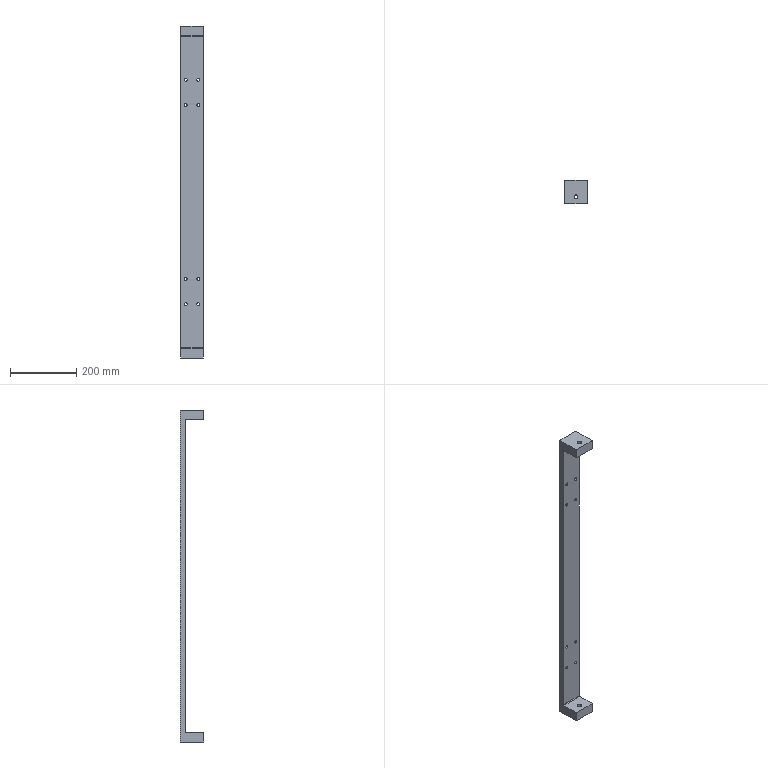Part | STEP file | Rear link plate | 1 solid | 32 faces | box 68 x 70 x 1000 mm | volume 1230922 mm3 | cylinder 22 | plane 10 | commonest cylinder face diameters 8.5 x16 12 x4 4 x2